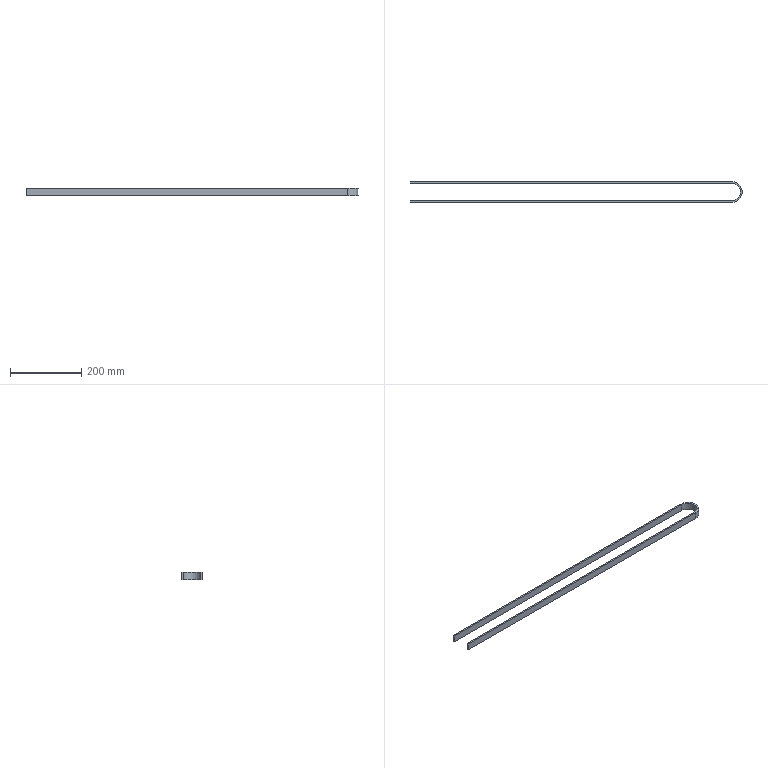Part | STEP file | Guide wheel mechanism revised.sldasm-Part-56 | 1 solid | 10 faces | box 931.5 x 59 x 20 mm | volume 170065 mm3 | plane 8 | cylinder 2 | commonest cylinder face diameters 50 x1 59 x1
STEP:
#1=CARTESIAN_POINT('',(1300.,25.,10.));
#2=VERTEX_POINT('',#1);
#3=CARTESIAN_POINT('',(1300.,25.,-10.));
#4=VERTEX_POINT('',#3);
#5=CARTESIAN_POINT('',(1300.,25.,10.));
#6=DIRECTION('',(0.,0.,-1.));
#7=VECTOR('',#6,1000.);
#8=LINE('',#5,#7);
#9=EDGE_CURVE('',#2,#4,#8,.T.);
#10=ORIENTED_EDGE('',*,*,#9,.T.);
#11=CARTESIAN_POINT('',(1300.,-25.,-10.));
#12=VERTEX_POINT('',#11);
#13=CARTESIAN_POINT('',(1300.,0.,-10.));
#14=DIRECTION('',(0.,0.,1.));
#15=DIRECTION('',(1.,0.,0.));
#16=AXIS2_PLACEMENT_3D('',#13,#14,#15);
#17=CIRCLE('',#16,25.);
#18=EDGE_CURVE('',#12,#4,#17,.T.);
#19=ORIENTED_EDGE('',*,*,#18,.F.);
#20=CARTESIAN_POINT('',(1300.,-25.,10.));
#21=VERTEX_POINT('',#20);
#22=CARTESIAN_POINT('',(1300.,-25.,10.));
#23=DIRECTION('',(0.,0.,-1.));
#24=VECTOR('',#23,1000.);
#25=LINE('',#22,#24);
#26=EDGE_CURVE('',#21,#12,#25,.T.);
#27=ORIENTED_EDGE('',*,*,#26,.F.);
#28=CARTESIAN_POINT('',(1300.,0.,10.));
#29=DIRECTION('',(0.,0.,1.));
#30=DIRECTION('',(1.,0.,0.));
#31=AXIS2_PLACEMENT_3D('',#28,#29,#30);
#32=CIRCLE('',#31,25.);
#33=EDGE_CURVE('',#21,#2,#32,.T.);
#34=ORIENTED_EDGE('',*,*,#33,.T.);
#35=EDGE_LOOP('',(#10,#19,#27,#34));
#36=FACE_OUTER_BOUND('',#35,.T.);
#37=CARTESIAN_POINT('',(1300.,0.,10.));
#38=DIRECTION('',(0.,0.,-1.));
#39=DIRECTION('',(-1.,0.,0.));
#40=AXIS2_PLACEMENT_3D('',#37,#38,#39);
#41=CYLINDRICAL_SURFACE('',#40,25.);
#42=ADVANCED_FACE('',(#36),#41,.F.);
#43=CARTESIAN_POINT('',(1300.,-29.5,10.));
#44=VERTEX_POINT('',#43);
#45=CARTESIAN_POINT('',(1300.,-29.5,-10.));
#46=VERTEX_POINT('',#45);
#47=CARTESIAN_POINT('',(1300.,-29.5,10.));
#48=DIRECTION('',(0.,0.,-1.));
#49=VECTOR('',#48,1000.);
#50=LINE('',#47,#49);
#51=EDGE_CURVE('',#44,#46,#50,.T.);
#52=ORIENTED_EDGE('',*,*,#51,.T.);
#53=CARTESIAN_POINT('',(1300.,29.5,-10.));
#54=VERTEX_POINT('',#53);
#55=CARTESIAN_POINT('',(1300.,0.,-10.));
#56=DIRECTION('',(0.,0.,1.));
#57=DIRECTION('',(1.,0.,0.));
#58=AXIS2_PLACEMENT_3D('',#55,#56,#57);
#59=CIRCLE('',#58,29.5);
#60=EDGE_CURVE('',#46,#54,#59,.T.);
#61=ORIENTED_EDGE('',*,*,#60,.T.);
#62=CARTESIAN_POINT('',(1300.,29.5,10.));
#63=VERTEX_POINT('',#62);
#64=CARTESIAN_POINT('',(1300.,29.5,10.));
#65=DIRECTION('',(0.,0.,-1.));
#66=VECTOR('',#65,1000.);
#67=LINE('',#64,#66);
#68=EDGE_CURVE('',#63,#54,#67,.T.);
#69=ORIENTED_EDGE('',*,*,#68,.F.);
#70=CARTESIAN_POINT('',(1300.,0.,10.));
#71=DIRECTION('',(0.,0.,1.));
#72=DIRECTION('',(1.,0.,0.));
#73=AXIS2_PLACEMENT_3D('',#70,#71,#72);
#74=CIRCLE('',#73,29.5);
#75=EDGE_CURVE('',#44,#63,#74,.T.);
#76=ORIENTED_EDGE('',*,*,#75,.F.);
#77=EDGE_LOOP('',(#52,#61,#69,#76));
#78=FACE_OUTER_BOUND('',#77,.T.);
#79=CARTESIAN_POINT('',(1300.,0.,10.));
#80=DIRECTION('',(0.,0.,-1.));
#81=DIRECTION('',(-1.,0.,0.));
#82=AXIS2_PLACEMENT_3D('',#79,#80,#81);
#83=CYLINDRICAL_SURFACE('',#82,29.5);
#84=ADVANCED_FACE('',(#78),#83,.T.);
#85=CARTESIAN_POINT('',(398.,-29.5,10.));
#86=VERTEX_POINT('',#85);
#87=CARTESIAN_POINT('',(398.,-25.,10.));
#88=VERTEX_POINT('',#87);
#89=CARTESIAN_POINT('',(398.,0.,10.));
#90=DIRECTION('',(0.,1.,0.));
#91=VECTOR('',#90,1000.);
#92=LINE('',#89,#91);
#93=EDGE_CURVE('',#86,#88,#92,.T.);
#94=ORIENTED_EDGE('',*,*,#93,.F.);
#95=CARTESIAN_POINT('',(0.,-29.5,10.));
#96=DIRECTION('',(1.,0.,0.));
#97=VECTOR('',#96,1000.);
#98=LINE('',#95,#97);
#99=EDGE_CURVE('',#86,#44,#98,.T.);
#100=ORIENTED_EDGE('',*,*,#99,.T.);
#101=ORIENTED_EDGE('',*,*,#75,.T.);
#102=CARTESIAN_POINT('',(398.,29.5,10.));
#103=VERTEX_POINT('',#102);
#104=CARTESIAN_POINT('',(1300.,29.5,10.));
#105=DIRECTION('',(-1.,0.,0.));
#106=VECTOR('',#105,1000.);
#107=LINE('',#104,#106);
#108=EDGE_CURVE('',#63,#103,#107,.T.);
#109=ORIENTED_EDGE('',*,*,#108,.T.);
#110=CARTESIAN_POINT('',(398.,25.,10.));
#111=VERTEX_POINT('',#110);
#112=CARTESIAN_POINT('',(398.,0.,10.));
#113=DIRECTION('',(0.,1.,0.));
#114=VECTOR('',#113,1000.);
#115=LINE('',#112,#114);
#116=EDGE_CURVE('',#111,#103,#115,.T.);
#117=ORIENTED_EDGE('',*,*,#116,.F.);
#118=CARTESIAN_POINT('',(1300.,25.,10.));
#119=DIRECTION('',(-1.,0.,0.));
#120=VECTOR('',#119,1000.);
#121=LINE('',#118,#120);
#122=EDGE_CURVE('',#2,#111,#121,.T.);
#123=ORIENTED_EDGE('',*,*,#122,.F.);
#124=ORIENTED_EDGE('',*,*,#33,.F.);
#125=CARTESIAN_POINT('',(0.,-25.,10.));
#126=DIRECTION('',(1.,0.,0.));
#127=VECTOR('',#126,1000.);
#128=LINE('',#125,#127);
#129=EDGE_CURVE('',#88,#21,#128,.T.);
#130=ORIENTED_EDGE('',*,*,#129,.F.);
#131=EDGE_LOOP('',(#94,#100,#101,#109,#117,#123,#124,#130));
#132=FACE_OUTER_BOUND('',#131,.T.);
#133=CARTESIAN_POINT('',(0.,0.,10.));
#134=DIRECTION('',(0.,0.,1.));
#135=DIRECTION('',(1.,0.,0.));
#136=AXIS2_PLACEMENT_3D('',#133,#134,#135);
#137=PLANE('',#136);
#138=ADVANCED_FACE('',(#132),#137,.T.);
#139=ORIENTED_EDGE('',*,*,#99,.F.);
#140=CARTESIAN_POINT('',(398.,-29.5,-10.));
#141=VERTEX_POINT('',#140);
#142=CARTESIAN_POINT('',(398.,-29.5,10.));
#143=DIRECTION('',(0.,0.,-1.));
#144=VECTOR('',#143,1000.);
#145=LINE('',#142,#144);
#146=EDGE_CURVE('',#86,#141,#145,.T.);
#147=ORIENTED_EDGE('',*,*,#146,.T.);
#148=CARTESIAN_POINT('',(0.,-29.5,-10.));
#149=DIRECTION('',(1.,0.,0.));
#150=VECTOR('',#149,1000.);
#151=LINE('',#148,#150);
#152=EDGE_CURVE('',#141,#46,#151,.T.);
#153=ORIENTED_EDGE('',*,*,#152,.T.);
#154=ORIENTED_EDGE('',*,*,#51,.F.);
#155=EDGE_LOOP('',(#139,#147,#153,#154));
#156=FACE_OUTER_BOUND('',#155,.T.);
#157=CARTESIAN_POINT('',(650.,-29.5,10.));
#158=DIRECTION('',(0.,1.,0.));
#159=DIRECTION('',(-1.,0.,0.));
#160=AXIS2_PLACEMENT_3D('',#157,#158,#159);
#161=PLANE('',#160);
#162=ADVANCED_FACE('',(#156),#161,.F.);
#163=CARTESIAN_POINT('',(398.,29.5,-10.));
#164=VERTEX_POINT('',#163);
#165=CARTESIAN_POINT('',(1300.,29.5,-10.));
#166=DIRECTION('',(-1.,0.,0.));
#167=VECTOR('',#166,1000.);
#168=LINE('',#165,#167);
#169=EDGE_CURVE('',#54,#164,#168,.T.);
#170=ORIENTED_EDGE('',*,*,#169,.T.);
#171=CARTESIAN_POINT('',(398.,29.5,-15.));
#172=DIRECTION('',(0.,0.,-1.));
#173=VECTOR('',#172,1000.);
#174=LINE('',#171,#173);
#175=EDGE_CURVE('',#103,#164,#174,.T.);
#176=ORIENTED_EDGE('',*,*,#175,.F.);
#177=ORIENTED_EDGE('',*,*,#108,.F.);
#178=ORIENTED_EDGE('',*,*,#68,.T.);
#179=EDGE_LOOP('',(#170,#176,#177,#178));
#180=FACE_OUTER_BOUND('',#179,.T.);
#181=CARTESIAN_POINT('',(1300.,29.5,10.));
#182=DIRECTION('',(0.,-1.,0.));
#183=DIRECTION('',(0.,0.,-1.));
#184=AXIS2_PLACEMENT_3D('',#181,#182,#183);
#185=PLANE('',#184);
#186=ADVANCED_FACE('',(#180),#185,.F.);
#187=CARTESIAN_POINT('',(398.,-25.,-10.));
#188=VERTEX_POINT('',#187);
#189=CARTESIAN_POINT('',(398.,-25.,10.));
#190=DIRECTION('',(0.,0.,-1.));
#191=VECTOR('',#190,1000.);
#192=LINE('',#189,#191);
#193=EDGE_CURVE('',#88,#188,#192,.T.);
#194=ORIENTED_EDGE('',*,*,#193,.F.);
#195=ORIENTED_EDGE('',*,*,#129,.T.);
#196=ORIENTED_EDGE('',*,*,#26,.T.);
#197=CARTESIAN_POINT('',(0.,-25.,-10.));
#198=DIRECTION('',(1.,0.,0.));
#199=VECTOR('',#198,1000.);
#200=LINE('',#197,#199);
#201=EDGE_CURVE('',#188,#12,#200,.T.);
#202=ORIENTED_EDGE('',*,*,#201,.F.);
#203=EDGE_LOOP('',(#194,#195,#196,#202));
#204=FACE_OUTER_BOUND('',#203,.T.);
#205=CARTESIAN_POINT('',(650.,-25.,10.));
#206=DIRECTION('',(0.,1.,0.));
#207=DIRECTION('',(-1.,0.,0.));
#208=AXIS2_PLACEMENT_3D('',#205,#206,#207);
#209=PLANE('',#208);
#210=ADVANCED_FACE('',(#204),#209,.T.);
#211=CARTESIAN_POINT('',(398.,25.,-10.));
#212=VERTEX_POINT('',#211);
#213=CARTESIAN_POINT('',(398.,25.,10.));
#214=DIRECTION('',(0.,0.,1.));
#215=VECTOR('',#214,1000.);
#216=LINE('',#213,#215);
#217=EDGE_CURVE('',#212,#111,#216,.T.);
#218=ORIENTED_EDGE('',*,*,#217,.F.);
#219=CARTESIAN_POINT('',(1300.,25.,-10.));
#220=DIRECTION('',(-1.,0.,0.));
#221=VECTOR('',#220,1000.);
#222=LINE('',#219,#221);
#223=EDGE_CURVE('',#4,#212,#222,.T.);
#224=ORIENTED_EDGE('',*,*,#223,.F.);
#225=ORIENTED_EDGE('',*,*,#9,.F.);
#226=ORIENTED_EDGE('',*,*,#122,.T.);
#227=EDGE_LOOP('',(#218,#224,#225,#226));
#228=FACE_OUTER_BOUND('',#227,.T.);
#229=CARTESIAN_POINT('',(1300.,25.,10.));
#230=DIRECTION('',(0.,-1.,0.));
#231=DIRECTION('',(0.,0.,-1.));
#232=AXIS2_PLACEMENT_3D('',#229,#230,#231);
#233=PLANE('',#232);
#234=ADVANCED_FACE('',(#228),#233,.T.);
#235=ORIENTED_EDGE('',*,*,#152,.F.);
#236=CARTESIAN_POINT('',(398.,0.,-10.));
#237=DIRECTION('',(0.,1.,0.));
#238=VECTOR('',#237,1000.);
#239=LINE('',#236,#238);
#240=EDGE_CURVE('',#141,#188,#239,.T.);
#241=ORIENTED_EDGE('',*,*,#240,.T.);
#242=ORIENTED_EDGE('',*,*,#201,.T.);
#243=ORIENTED_EDGE('',*,*,#18,.T.);
#244=ORIENTED_EDGE('',*,*,#223,.T.);
#245=CARTESIAN_POINT('',(398.,0.,-10.));
#246=DIRECTION('',(0.,1.,0.));
#247=VECTOR('',#246,1000.);
#248=LINE('',#245,#247);
#249=EDGE_CURVE('',#212,#164,#248,.T.);
#250=ORIENTED_EDGE('',*,*,#249,.T.);
#251=ORIENTED_EDGE('',*,*,#169,.F.);
#252=ORIENTED_EDGE('',*,*,#60,.F.);
#253=EDGE_LOOP('',(#235,#241,#242,#243,#244,#250,#251,#252));
#254=FACE_OUTER_BOUND('',#253,.T.);
#255=CARTESIAN_POINT('',(0.,0.,-10.));
#256=DIRECTION('',(0.,0.,1.));
#257=DIRECTION('',(1.,0.,0.));
#258=AXIS2_PLACEMENT_3D('',#255,#256,#257);
#259=PLANE('',#258);
#260=ADVANCED_FACE('',(#254),#259,.F.);
#261=ORIENTED_EDGE('',*,*,#217,.T.);
#262=ORIENTED_EDGE('',*,*,#116,.T.);
#263=ORIENTED_EDGE('',*,*,#175,.T.);
#264=ORIENTED_EDGE('',*,*,#249,.F.);
#265=EDGE_LOOP('',(#261,#262,#263,#264));
#266=FACE_OUTER_BOUND('',#265,.T.);
#267=CARTESIAN_POINT('',(398.,-30.5,-15.));
#268=DIRECTION('',(1.,0.,0.));
#269=DIRECTION('',(0.,0.,-1.));
#270=AXIS2_PLACEMENT_3D('',#267,#268,#269);
#271=PLANE('',#270);
#272=ADVANCED_FACE('',(#266),#271,.F.);
#273=ORIENTED_EDGE('',*,*,#146,.F.);
#274=ORIENTED_EDGE('',*,*,#93,.T.);
#275=ORIENTED_EDGE('',*,*,#193,.T.);
#276=ORIENTED_EDGE('',*,*,#240,.F.);
#277=EDGE_LOOP('',(#273,#274,#275,#276));
#278=FACE_OUTER_BOUND('',#277,.T.);
#279=CARTESIAN_POINT('',(398.,-30.5,-15.));
#280=DIRECTION('',(1.,0.,0.));
#281=DIRECTION('',(0.,0.,-1.));
#282=AXIS2_PLACEMENT_3D('',#279,#280,#281);
#283=PLANE('',#282);
#284=ADVANCED_FACE('',(#278),#283,.F.);
#285=CLOSED_SHELL('',(#42,#84,#138,#162,#186,#210,#234,#260,#272,#284));
#286=MANIFOLD_SOLID_BREP('',#285);
#287=CARTESIAN_POINT('',(0.,0.,0.));
#288=DIRECTION('',(0.,0.,1.));
#289=DIRECTION('',(1.,0.,0.));
#290=AXIS2_PLACEMENT_3D('',#287,#288,#289);
#291=(LENGTH_UNIT()NAMED_UNIT(*)SI_UNIT(.MILLI.,.METRE.));
#292=UNCERTAINTY_MEASURE_WITH_UNIT(LENGTH_MEASURE(0.00001),#291,'','');
#293=(NAMED_UNIT(*)PLANE_ANGLE_UNIT()SI_UNIT($,.RADIAN.));
#294=(NAMED_UNIT(*)SI_UNIT($,.STERADIAN.)SOLID_ANGLE_UNIT());
#295=(GEOMETRIC_REPRESENTATION_CONTEXT(3)GLOBAL_UNCERTAINTY_ASSIGNED_CONTEXT((#292))GLOBAL_UNIT_ASSIGNED_CONTEXT((#291,#293,#294))REPRESENTATION_CONTEXT('',''));
#296=ADVANCED_BREP_SHAPE_REPRESENTATION('',(#286,#290),#295);